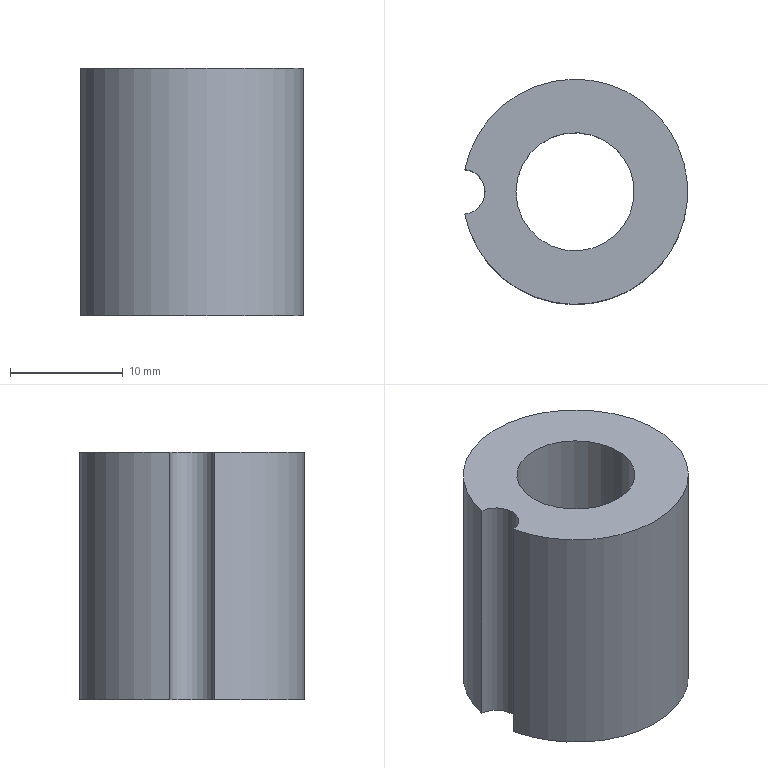Part | NX | features solid 2 | 1 solid | 7 faces | box 19.8 x 20 x 22 mm | volume 4341 mm3 | cylinder 4 | plane 3 | commonest cylinder face diameters 4 x1 10.5 x1 12.6 x1 20 x1
STEP:
#1=CARTESIAN_POINT('',(-747.3,186.01,29.));
#2=VERTEX_POINT('',#1);
#3=CARTESIAN_POINT('',(-747.3,189.99,29.));
#4=VERTEX_POINT('',#3);
#5=CARTESIAN_POINT('',(-747.5,188.,29.));
#6=DIRECTION('',(0.,0.,1.));
#7=DIRECTION('',(0.,1.,0.));
#8=AXIS2_PLACEMENT_3D('',#5,#6,#7);
#9=CIRCLE('',#8,2.);
#10=EDGE_CURVE('',#2,#4,#9,.T.);
#11=ORIENTED_EDGE('',*,*,#10,.T.);
#12=CARTESIAN_POINT('',(-737.5,188.,29.));
#13=DIRECTION('',(0.,0.,1.));
#14=DIRECTION('',(1.,0.,0.));
#15=AXIS2_PLACEMENT_3D('',#12,#13,#14);
#16=CIRCLE('',#15,10.);
#17=EDGE_CURVE('',#2,#4,#16,.T.);
#18=ORIENTED_EDGE('',*,*,#17,.F.);
#19=EDGE_LOOP('',(#11,#18));
#20=FACE_BOUND('',#19,.T.);
#21=CARTESIAN_POINT('',(-731.2,188.,29.));
#22=VERTEX_POINT('',#21);
#23=CARTESIAN_POINT('',(-737.5,188.,29.));
#24=DIRECTION('',(0.,0.,1.));
#25=DIRECTION('',(1.,0.,0.));
#26=AXIS2_PLACEMENT_3D('',#23,#24,#25);
#27=CIRCLE('',#26,6.3);
#28=EDGE_CURVE('',#22,#22,#27,.F.);
#29=ORIENTED_EDGE('',*,*,#28,.F.);
#30=EDGE_LOOP('',(#29));
#31=FACE_BOUND('',#30,.T.);
#32=CARTESIAN_POINT('',(-737.5,188.,29.));
#33=DIRECTION('',(0.,0.,-1.));
#34=DIRECTION('',(0.,-1.,0.));
#35=AXIS2_PLACEMENT_3D('',#32,#33,#34);
#36=PLANE('',#35);
#37=ADVANCED_FACE('',(#20,#31),#36,.T.);
#38=CARTESIAN_POINT('',(-747.3,189.99,51.));
#39=VERTEX_POINT('',#38);
#40=CARTESIAN_POINT('',(-747.3,186.01,51.));
#41=VERTEX_POINT('',#40);
#42=CARTESIAN_POINT('',(-747.5,188.,51.));
#43=DIRECTION('',(0.,0.,-1.));
#44=DIRECTION('',(0.,-1.,0.));
#45=AXIS2_PLACEMENT_3D('',#42,#43,#44);
#46=CIRCLE('',#45,2.);
#47=EDGE_CURVE('',#39,#41,#46,.T.);
#48=ORIENTED_EDGE('',*,*,#47,.T.);
#49=CARTESIAN_POINT('',(-737.5,188.,51.));
#50=DIRECTION('',(0.,0.,-1.));
#51=DIRECTION('',(-1.,0.,0.));
#52=AXIS2_PLACEMENT_3D('',#49,#50,#51);
#53=CIRCLE('',#52,10.);
#54=EDGE_CURVE('',#39,#41,#53,.T.);
#55=ORIENTED_EDGE('',*,*,#54,.F.);
#56=EDGE_LOOP('',(#48,#55));
#57=FACE_BOUND('',#56,.T.);
#58=CARTESIAN_POINT('',(-742.75,188.,51.));
#59=VERTEX_POINT('',#58);
#60=CARTESIAN_POINT('',(-737.5,188.,51.));
#61=DIRECTION('',(0.,0.,-1.));
#62=DIRECTION('',(-1.,0.,0.));
#63=AXIS2_PLACEMENT_3D('',#60,#61,#62);
#64=CIRCLE('',#63,5.25);
#65=EDGE_CURVE('',#59,#59,#64,.F.);
#66=ORIENTED_EDGE('',*,*,#65,.F.);
#67=EDGE_LOOP('',(#66));
#68=FACE_BOUND('',#67,.T.);
#69=CARTESIAN_POINT('',(-737.5,188.,51.));
#70=DIRECTION('',(0.,0.,1.));
#71=DIRECTION('',(0.,1.,0.));
#72=AXIS2_PLACEMENT_3D('',#69,#70,#71);
#73=PLANE('',#72);
#74=ADVANCED_FACE('',(#57,#68),#73,.T.);
#75=CARTESIAN_POINT('',(-747.3,186.01,40.));
#76=DIRECTION('',(0.,0.,-1.));
#77=VECTOR('',#76,1000.);
#78=LINE('',#75,#77);
#79=EDGE_CURVE('',#41,#2,#78,.T.);
#80=ORIENTED_EDGE('',*,*,#79,.T.);
#81=ORIENTED_EDGE('',*,*,#17,.T.);
#82=CARTESIAN_POINT('',(-747.3,189.99,40.));
#83=DIRECTION('',(0.,0.,-1.));
#84=VECTOR('',#83,1000.);
#85=LINE('',#82,#84);
#86=EDGE_CURVE('',#4,#39,#85,.F.);
#87=ORIENTED_EDGE('',*,*,#86,.T.);
#88=ORIENTED_EDGE('',*,*,#54,.T.);
#89=EDGE_LOOP('',(#80,#81,#87,#88));
#90=FACE_BOUND('',#89,.T.);
#91=CARTESIAN_POINT('',(-737.5,188.,51.));
#92=DIRECTION('',(0.,0.,-1.));
#93=DIRECTION('',(0.,-1.,0.));
#94=AXIS2_PLACEMENT_3D('',#91,#92,#93);
#95=CYLINDRICAL_SURFACE('',#94,10.);
#96=ADVANCED_FACE('',(#90),#95,.T.);
#97=CARTESIAN_POINT('',(-742.75,188.,43.));
#98=VERTEX_POINT('',#97);
#99=CARTESIAN_POINT('',(-737.5,188.,43.));
#100=DIRECTION('',(0.,0.,-1.));
#101=DIRECTION('',(-1.,0.,0.));
#102=AXIS2_PLACEMENT_3D('',#99,#100,#101);
#103=CIRCLE('',#102,5.25);
#104=EDGE_CURVE('',#98,#98,#103,.T.);
#105=ORIENTED_EDGE('',*,*,#104,.T.);
#106=EDGE_LOOP('',(#105));
#107=FACE_BOUND('',#106,.T.);
#108=ORIENTED_EDGE('',*,*,#65,.T.);
#109=EDGE_LOOP('',(#108));
#110=FACE_BOUND('',#109,.T.);
#111=CARTESIAN_POINT('',(-737.5,188.,52.));
#112=DIRECTION('',(0.,0.,-1.));
#113=DIRECTION('',(0.,-1.,0.));
#114=AXIS2_PLACEMENT_3D('',#111,#112,#113);
#115=CYLINDRICAL_SURFACE('',#114,5.25);
#116=ADVANCED_FACE('',(#107,#110),#115,.F.);
#117=CARTESIAN_POINT('',(-743.8,188.,43.));
#118=VERTEX_POINT('',#117);
#119=CARTESIAN_POINT('',(-737.5,188.,43.));
#120=DIRECTION('',(0.,0.,-1.));
#121=DIRECTION('',(-1.,0.,0.));
#122=AXIS2_PLACEMENT_3D('',#119,#120,#121);
#123=CIRCLE('',#122,6.3);
#124=EDGE_CURVE('',#118,#118,#123,.T.);
#125=ORIENTED_EDGE('',*,*,#124,.T.);
#126=EDGE_LOOP('',(#125));
#127=FACE_BOUND('',#126,.T.);
#128=ORIENTED_EDGE('',*,*,#104,.F.);
#129=EDGE_LOOP('',(#128));
#130=FACE_BOUND('',#129,.T.);
#131=CARTESIAN_POINT('',(-737.5,188.,43.));
#132=DIRECTION('',(0.,0.,1.));
#133=DIRECTION('',(0.,1.,0.));
#134=AXIS2_PLACEMENT_3D('',#131,#132,#133);
#135=PLANE('',#134);
#136=ADVANCED_FACE('',(#127,#130),#135,.F.);
#137=ORIENTED_EDGE('',*,*,#28,.T.);
#138=EDGE_LOOP('',(#137));
#139=FACE_BOUND('',#138,.T.);
#140=ORIENTED_EDGE('',*,*,#124,.F.);
#141=EDGE_LOOP('',(#140));
#142=FACE_BOUND('',#141,.T.);
#143=CARTESIAN_POINT('',(-737.5,188.,43.));
#144=DIRECTION('',(0.,0.,-1.));
#145=DIRECTION('',(0.,-1.,0.));
#146=AXIS2_PLACEMENT_3D('',#143,#144,#145);
#147=CYLINDRICAL_SURFACE('',#146,6.3);
#148=ADVANCED_FACE('',(#139,#142),#147,.F.);
#149=ORIENTED_EDGE('',*,*,#79,.F.);
#150=ORIENTED_EDGE('',*,*,#47,.F.);
#151=ORIENTED_EDGE('',*,*,#86,.F.);
#152=ORIENTED_EDGE('',*,*,#10,.F.);
#153=EDGE_LOOP('',(#149,#150,#151,#152));
#154=FACE_BOUND('',#153,.T.);
#155=CARTESIAN_POINT('',(-747.5,188.,51.));
#156=DIRECTION('',(0.,0.,-1.));
#157=DIRECTION('',(0.,-1.,0.));
#158=AXIS2_PLACEMENT_3D('',#155,#156,#157);
#159=CYLINDRICAL_SURFACE('',#158,2.);
#160=ADVANCED_FACE('',(#154),#159,.F.);
#161=CLOSED_SHELL('',(#37,#74,#96,#116,#136,#148,#160));
#162=MANIFOLD_SOLID_BREP('',#161);
#163=(LENGTH_UNIT()NAMED_UNIT(*)SI_UNIT(.MILLI.,.METRE.));
#164=UNCERTAINTY_MEASURE_WITH_UNIT(LENGTH_MEASURE(0.00001),#163,'','');
#165=(NAMED_UNIT(*)PLANE_ANGLE_UNIT()SI_UNIT($,.RADIAN.));
#166=(NAMED_UNIT(*)SI_UNIT($,.STERADIAN.)SOLID_ANGLE_UNIT());
#167=(GEOMETRIC_REPRESENTATION_CONTEXT(3)GLOBAL_UNCERTAINTY_ASSIGNED_CONTEXT((#164))GLOBAL_UNIT_ASSIGNED_CONTEXT((#163,#165,#166))REPRESENTATION_CONTEXT('',''));
#168=ADVANCED_BREP_SHAPE_REPRESENTATION('',(#162),#167);